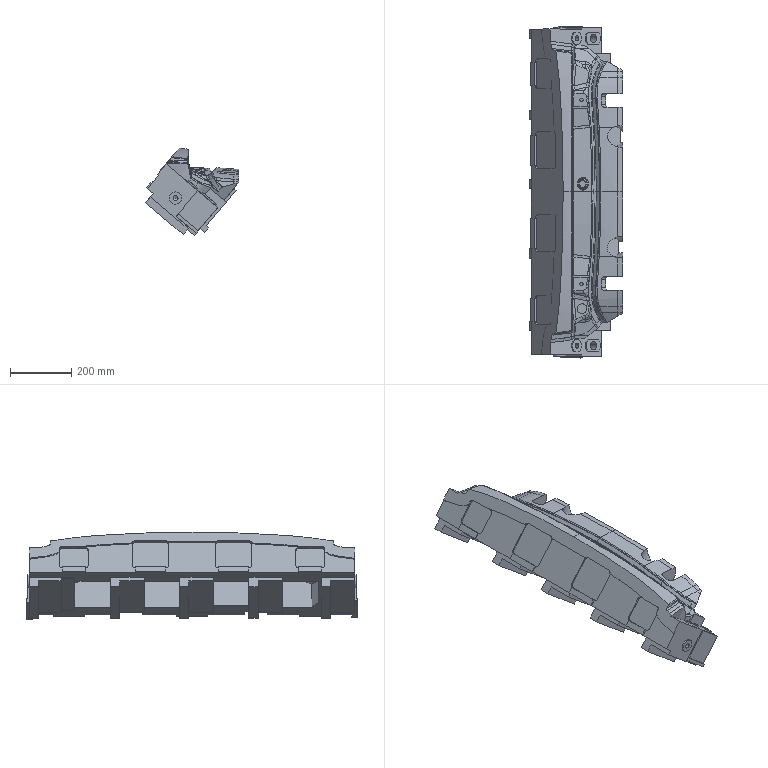Part | NX | features solid 2 | 1 solid | 478 faces | box 302.895 x 1080 x 284.062 mm | volume 32585041 mm3 | spline 259 | plane 160 | cylinder 51 | sphere 4 | cone 4 | commonest cylinder face diameters 20 x35 16 x4 40 x4 60 x4 27 x2 70 x2